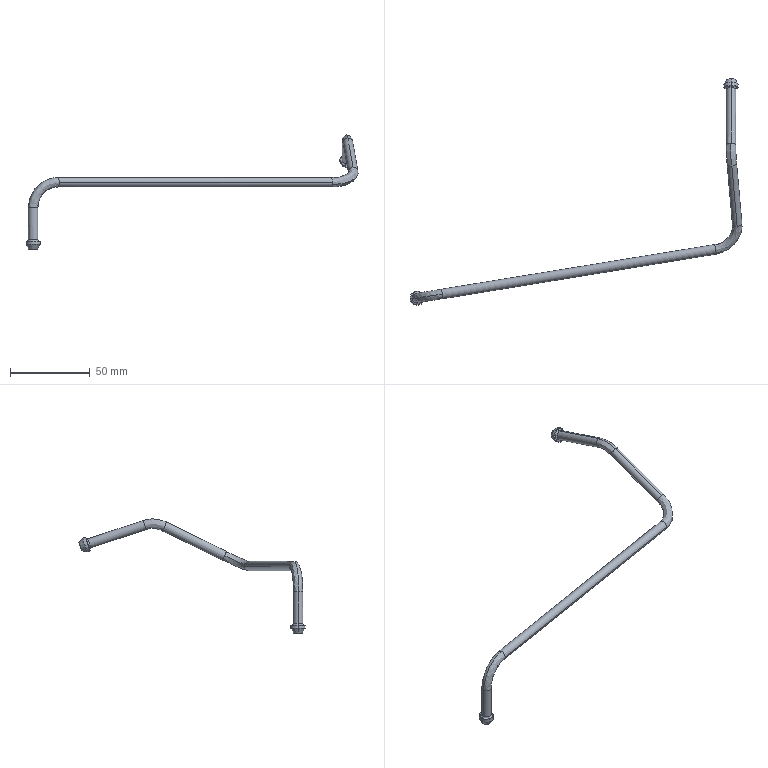Part | SolidWorks | features BaseBody 1 | 1 solid | 56 faces | box 208.375 x 142.113 x 71.742 mm | volume 9302 mm3 | cylinder 24 | spline 16 | cone 12 | plane 4 | commonest cylinder face diameters 1.6 x8 6 x8 2 x4 9 x4